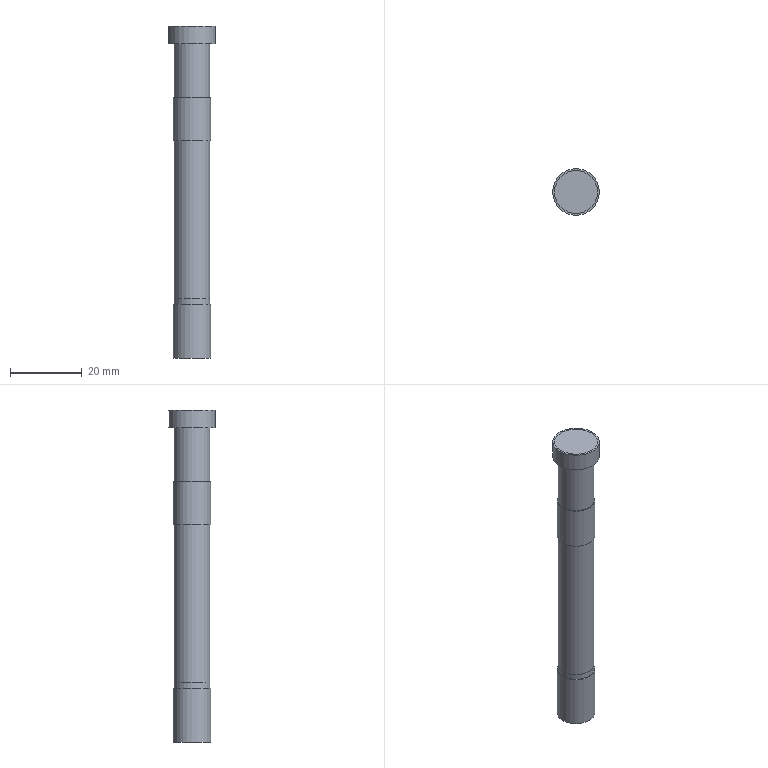Part | NX | features BREP 2 | 2 solids | 17 faces | box 13 x 13 x 92.6 mm | volume 14175 mm3 | plane 9 | cylinder 7 | cone 1 | commonest cylinder face diameters 10 x3 10.5 x2 12 x1 13 x1
STEP:
#1=CARTESIAN_POINT('',(6.5,0.,-5.));
#2=VERTEX_POINT('',#1);
#3=CARTESIAN_POINT('',(0.,0.,-5.));
#4=DIRECTION('',(0.,0.,1.));
#5=DIRECTION('',(1.,0.,0.));
#6=AXIS2_PLACEMENT_3D('',#3,#4,#5);
#7=CIRCLE('',#6,6.5);
#8=EDGE_CURVE('',#2,#2,#7,.T.);
#9=ORIENTED_EDGE('',*,*,#8,.T.);
#10=EDGE_LOOP('',(#9));
#11=FACE_BOUND('',#10,.T.);
#12=CARTESIAN_POINT('',(6.5,0.,0.));
#13=VERTEX_POINT('',#12);
#14=CARTESIAN_POINT('',(0.,0.,0.));
#15=DIRECTION('',(0.,0.,1.));
#16=DIRECTION('',(1.,0.,0.));
#17=AXIS2_PLACEMENT_3D('',#14,#15,#16);
#18=CIRCLE('',#17,6.5);
#19=EDGE_CURVE('',#13,#13,#18,.T.);
#20=ORIENTED_EDGE('',*,*,#19,.F.);
#21=EDGE_LOOP('',(#20));
#22=FACE_BOUND('',#21,.T.);
#23=CARTESIAN_POINT('',(0.,0.,-5.));
#24=DIRECTION('',(0.,0.,1.));
#25=DIRECTION('',(-1.,0.,0.));
#26=AXIS2_PLACEMENT_3D('',#23,#24,#25);
#27=CYLINDRICAL_SURFACE('',#26,6.5);
#28=ADVANCED_FACE('',(#11,#22),#27,.T.);
#29=CARTESIAN_POINT('',(-5.,0.,-5.));
#30=VERTEX_POINT('',#29);
#31=CARTESIAN_POINT('',(0.,0.,-5.));
#32=DIRECTION('',(0.,0.,-1.));
#33=DIRECTION('',(-1.,0.,0.));
#34=AXIS2_PLACEMENT_3D('',#31,#32,#33);
#35=CIRCLE('',#34,5.);
#36=EDGE_CURVE('',#30,#30,#35,.T.);
#37=ORIENTED_EDGE('',*,*,#36,.F.);
#38=EDGE_LOOP('',(#37));
#39=FACE_BOUND('',#38,.T.);
#40=ORIENTED_EDGE('',*,*,#8,.F.);
#41=EDGE_LOOP('',(#40));
#42=FACE_BOUND('',#41,.T.);
#43=CARTESIAN_POINT('',(0.,0.,-5.));
#44=DIRECTION('',(0.,0.,1.));
#45=DIRECTION('',(-1.,0.,0.));
#46=AXIS2_PLACEMENT_3D('',#43,#44,#45);
#47=PLANE('',#46);
#48=ADVANCED_FACE('',(#39,#42),#47,.F.);
#49=ORIENTED_EDGE('',*,*,#19,.T.);
#50=EDGE_LOOP('',(#49));
#51=FACE_BOUND('',#50,.T.);
#52=CARTESIAN_POINT('',(0.,0.,0.));
#53=DIRECTION('',(0.,0.,1.));
#54=DIRECTION('',(-1.,0.,0.));
#55=AXIS2_PLACEMENT_3D('',#52,#53,#54);
#56=PLANE('',#55);
#57=ADVANCED_FACE('',(#51),#56,.T.);
#58=CARTESIAN_POINT('',(-5.,0.,-20.));
#59=VERTEX_POINT('',#58);
#60=CARTESIAN_POINT('',(0.,0.,-20.));
#61=DIRECTION('',(0.,0.,-1.));
#62=DIRECTION('',(-1.,0.,0.));
#63=AXIS2_PLACEMENT_3D('',#60,#61,#62);
#64=CIRCLE('',#63,5.);
#65=EDGE_CURVE('',#59,#59,#64,.T.);
#66=ORIENTED_EDGE('',*,*,#65,.F.);
#67=EDGE_LOOP('',(#66));
#68=FACE_BOUND('',#67,.T.);
#69=ORIENTED_EDGE('',*,*,#36,.T.);
#70=EDGE_LOOP('',(#69));
#71=FACE_BOUND('',#70,.T.);
#72=CARTESIAN_POINT('',(0.,0.,-5.));
#73=DIRECTION('',(0.,0.,-1.));
#74=DIRECTION('',(1.,0.,0.));
#75=AXIS2_PLACEMENT_3D('',#72,#73,#74);
#76=CYLINDRICAL_SURFACE('',#75,5.);
#77=ADVANCED_FACE('',(#68,#71),#76,.T.);
#78=CARTESIAN_POINT('',(-5.,0.,-32.));
#79=VERTEX_POINT('',#78);
#80=CARTESIAN_POINT('',(0.,0.,-32.));
#81=DIRECTION('',(0.,0.,-1.));
#82=DIRECTION('',(-1.,0.,0.));
#83=AXIS2_PLACEMENT_3D('',#80,#81,#82);
#84=CIRCLE('',#83,5.);
#85=EDGE_CURVE('',#79,#79,#84,.T.);
#86=ORIENTED_EDGE('',*,*,#85,.F.);
#87=EDGE_LOOP('',(#86));
#88=FACE_BOUND('',#87,.T.);
#89=CARTESIAN_POINT('',(-5.25,0.,-32.));
#90=VERTEX_POINT('',#89);
#91=CARTESIAN_POINT('',(0.,0.,-32.));
#92=DIRECTION('',(0.,0.,-1.));
#93=DIRECTION('',(-1.,0.,0.));
#94=AXIS2_PLACEMENT_3D('',#91,#92,#93);
#95=CIRCLE('',#94,5.25);
#96=EDGE_CURVE('',#90,#90,#95,.T.);
#97=ORIENTED_EDGE('',*,*,#96,.T.);
#98=EDGE_LOOP('',(#97));
#99=FACE_BOUND('',#98,.T.);
#100=CARTESIAN_POINT('',(0.,0.,-32.));
#101=DIRECTION('',(0.,0.,-1.));
#102=DIRECTION('',(1.,0.,0.));
#103=AXIS2_PLACEMENT_3D('',#100,#101,#102);
#104=PLANE('',#103);
#105=ADVANCED_FACE('',(#88,#99),#104,.T.);
#106=ORIENTED_EDGE('',*,*,#65,.T.);
#107=EDGE_LOOP('',(#106));
#108=FACE_BOUND('',#107,.T.);
#109=CARTESIAN_POINT('',(-5.25,0.,-20.));
#110=VERTEX_POINT('',#109);
#111=CARTESIAN_POINT('',(0.,0.,-20.));
#112=DIRECTION('',(0.,0.,-1.));
#113=DIRECTION('',(-1.,0.,0.));
#114=AXIS2_PLACEMENT_3D('',#111,#112,#113);
#115=CIRCLE('',#114,5.25);
#116=EDGE_CURVE('',#110,#110,#115,.T.);
#117=ORIENTED_EDGE('',*,*,#116,.F.);
#118=EDGE_LOOP('',(#117));
#119=FACE_BOUND('',#118,.T.);
#120=CARTESIAN_POINT('',(0.,0.,-20.));
#121=DIRECTION('',(0.,0.,1.));
#122=DIRECTION('',(-1.,0.,0.));
#123=AXIS2_PLACEMENT_3D('',#120,#121,#122);
#124=PLANE('',#123);
#125=ADVANCED_FACE('',(#108,#119),#124,.T.);
#126=ORIENTED_EDGE('',*,*,#96,.F.);
#127=EDGE_LOOP('',(#126));
#128=FACE_BOUND('',#127,.T.);
#129=ORIENTED_EDGE('',*,*,#116,.T.);
#130=EDGE_LOOP('',(#129));
#131=FACE_BOUND('',#130,.T.);
#132=CARTESIAN_POINT('',(0.,0.,-20.));
#133=DIRECTION('',(0.,0.,-1.));
#134=DIRECTION('',(1.,0.,0.));
#135=AXIS2_PLACEMENT_3D('',#132,#133,#134);
#136=CYLINDRICAL_SURFACE('',#135,5.25);
#137=ADVANCED_FACE('',(#128,#131),#136,.T.);
#138=CARTESIAN_POINT('',(-5.,0.,-77.6));
#139=VERTEX_POINT('',#138);
#140=CARTESIAN_POINT('',(0.,0.,-77.6));
#141=DIRECTION('',(0.,0.,-1.));
#142=DIRECTION('',(-1.,0.,0.));
#143=AXIS2_PLACEMENT_3D('',#140,#141,#142);
#144=CIRCLE('',#143,5.);
#145=EDGE_CURVE('',#139,#139,#144,.T.);
#146=ORIENTED_EDGE('',*,*,#145,.F.);
#147=EDGE_LOOP('',(#146));
#148=FACE_BOUND('',#147,.T.);
#149=ORIENTED_EDGE('',*,*,#85,.T.);
#150=EDGE_LOOP('',(#149));
#151=FACE_BOUND('',#150,.T.);
#152=CARTESIAN_POINT('',(0.,0.,-32.));
#153=DIRECTION('',(0.,0.,-1.));
#154=DIRECTION('',(1.,0.,0.));
#155=AXIS2_PLACEMENT_3D('',#152,#153,#154);
#156=CYLINDRICAL_SURFACE('',#155,5.);
#157=ADVANCED_FACE('',(#148,#151),#156,.T.);
#158=CARTESIAN_POINT('',(-5.25,0.,-92.6));
#159=VERTEX_POINT('',#158);
#160=CARTESIAN_POINT('',(0.,0.,-92.6));
#161=DIRECTION('',(0.,0.,-1.));
#162=DIRECTION('',(-1.,0.,0.));
#163=AXIS2_PLACEMENT_3D('',#160,#161,#162);
#164=CIRCLE('',#163,5.25);
#165=EDGE_CURVE('',#159,#159,#164,.T.);
#166=ORIENTED_EDGE('',*,*,#165,.T.);
#167=EDGE_LOOP('',(#166));
#168=FACE_BOUND('',#167,.T.);
#169=CARTESIAN_POINT('',(0.,0.,-92.6));
#170=DIRECTION('',(0.,0.,-1.));
#171=DIRECTION('',(1.,0.,0.));
#172=AXIS2_PLACEMENT_3D('',#169,#170,#171);
#173=PLANE('',#172);
#174=ADVANCED_FACE('',(#168),#173,.T.);
#175=ORIENTED_EDGE('',*,*,#145,.T.);
#176=EDGE_LOOP('',(#175));
#177=FACE_BOUND('',#176,.T.);
#178=CARTESIAN_POINT('',(-5.25,0.,-77.6));
#179=VERTEX_POINT('',#178);
#180=CARTESIAN_POINT('',(0.,0.,-77.6));
#181=DIRECTION('',(0.,0.,-1.));
#182=DIRECTION('',(-1.,0.,0.));
#183=AXIS2_PLACEMENT_3D('',#180,#181,#182);
#184=CIRCLE('',#183,5.25);
#185=EDGE_CURVE('',#179,#179,#184,.T.);
#186=ORIENTED_EDGE('',*,*,#185,.F.);
#187=EDGE_LOOP('',(#186));
#188=FACE_BOUND('',#187,.T.);
#189=CARTESIAN_POINT('',(0.,0.,-77.6));
#190=DIRECTION('',(0.,0.,1.));
#191=DIRECTION('',(-1.,0.,0.));
#192=AXIS2_PLACEMENT_3D('',#189,#190,#191);
#193=PLANE('',#192);
#194=ADVANCED_FACE('',(#177,#188),#193,.T.);
#195=ORIENTED_EDGE('',*,*,#165,.F.);
#196=EDGE_LOOP('',(#195));
#197=FACE_BOUND('',#196,.T.);
#198=ORIENTED_EDGE('',*,*,#185,.T.);
#199=EDGE_LOOP('',(#198));
#200=FACE_BOUND('',#199,.T.);
#201=CARTESIAN_POINT('',(0.,0.,-77.6));
#202=DIRECTION('',(0.,0.,-1.));
#203=DIRECTION('',(1.,0.,0.));
#204=AXIS2_PLACEMENT_3D('',#201,#202,#203);
#205=CYLINDRICAL_SURFACE('',#204,5.25);
#206=ADVANCED_FACE('',(#197,#200),#205,.T.);
#207=CLOSED_SHELL('',(#28,#48,#57,#77,#105,#125,#137,#157,#174,#194,#206));
#208=MANIFOLD_SOLID_BREP('',#207);
#209=CARTESIAN_POINT('',(6.,0.,-5.));
#210=VERTEX_POINT('',#209);
#211=CARTESIAN_POINT('',(0.,0.,-5.));
#212=DIRECTION('',(0.,0.,1.));
#213=DIRECTION('',(1.,0.,0.));
#214=AXIS2_PLACEMENT_3D('',#211,#212,#213);
#215=CIRCLE('',#214,6.);
#216=EDGE_CURVE('',#210,#210,#215,.T.);
#217=ORIENTED_EDGE('',*,*,#216,.T.);
#218=EDGE_LOOP('',(#217));
#219=FACE_BOUND('',#218,.T.);
#220=CARTESIAN_POINT('',(6.,0.,0.));
#221=VERTEX_POINT('',#220);
#222=CARTESIAN_POINT('',(0.,0.,0.));
#223=DIRECTION('',(0.,0.,1.));
#224=DIRECTION('',(1.,0.,0.));
#225=AXIS2_PLACEMENT_3D('',#222,#223,#224);
#226=CIRCLE('',#225,6.);
#227=EDGE_CURVE('',#221,#221,#226,.T.);
#228=ORIENTED_EDGE('',*,*,#227,.F.);
#229=EDGE_LOOP('',(#228));
#230=FACE_BOUND('',#229,.T.);
#231=CARTESIAN_POINT('',(0.,0.,-5.));
#232=DIRECTION('',(0.,0.,1.));
#233=DIRECTION('',(-1.,0.,0.));
#234=AXIS2_PLACEMENT_3D('',#231,#232,#233);
#235=CYLINDRICAL_SURFACE('',#234,6.);
#236=ADVANCED_FACE('',(#219,#230),#235,.T.);
#237=CARTESIAN_POINT('',(-5.,0.,-5.));
#238=VERTEX_POINT('',#237);
#239=CARTESIAN_POINT('',(0.,0.,-5.));
#240=DIRECTION('',(0.,0.,-1.));
#241=DIRECTION('',(-1.,0.,0.));
#242=AXIS2_PLACEMENT_3D('',#239,#240,#241);
#243=CIRCLE('',#242,5.);
#244=EDGE_CURVE('',#238,#238,#243,.T.);
#245=ORIENTED_EDGE('',*,*,#244,.F.);
#246=EDGE_LOOP('',(#245));
#247=FACE_BOUND('',#246,.T.);
#248=ORIENTED_EDGE('',*,*,#216,.F.);
#249=EDGE_LOOP('',(#248));
#250=FACE_BOUND('',#249,.T.);
#251=CARTESIAN_POINT('',(0.,0.,-5.));
#252=DIRECTION('',(0.,0.,1.));
#253=DIRECTION('',(-1.,0.,0.));
#254=AXIS2_PLACEMENT_3D('',#251,#252,#253);
#255=PLANE('',#254);
#256=ADVANCED_FACE('',(#247,#250),#255,.F.);
#257=ORIENTED_EDGE('',*,*,#227,.T.);
#258=EDGE_LOOP('',(#257));
#259=FACE_BOUND('',#258,.T.);
#260=CARTESIAN_POINT('',(0.,0.,0.));
#261=DIRECTION('',(0.,0.,1.));
#262=DIRECTION('',(-1.,0.,0.));
#263=AXIS2_PLACEMENT_3D('',#260,#261,#262);
#264=PLANE('',#263);
#265=ADVANCED_FACE('',(#259),#264,.T.);
#266=CARTESIAN_POINT('',(-4.295,0.,-80.));
#267=VERTEX_POINT('',#266);
#268=CARTESIAN_POINT('',(0.,0.,-80.));
#269=DIRECTION('',(0.,0.,-1.));
#270=DIRECTION('',(-1.,0.,0.));
#271=AXIS2_PLACEMENT_3D('',#268,#269,#270);
#272=CIRCLE('',#271,4.295);
#273=EDGE_CURVE('',#267,#267,#272,.T.);
#274=ORIENTED_EDGE('',*,*,#273,.T.);
#275=EDGE_LOOP('',(#274));
#276=FACE_BOUND('',#275,.T.);
#277=CARTESIAN_POINT('',(0.,0.,-80.));
#278=DIRECTION('',(0.,0.,-1.));
#279=DIRECTION('',(1.,0.,0.));
#280=AXIS2_PLACEMENT_3D('',#277,#278,#279);
#281=PLANE('',#280);
#282=ADVANCED_FACE('',(#276),#281,.T.);
#283=CARTESIAN_POINT('',(-5.,0.,-76.));
#284=VERTEX_POINT('',#283);
#285=CARTESIAN_POINT('',(0.,0.,-76.));
#286=DIRECTION('',(0.,0.,1.));
#287=DIRECTION('',(-1.,0.,0.));
#288=AXIS2_PLACEMENT_3D('',#285,#286,#287);
#289=CIRCLE('',#288,5.);
#290=EDGE_CURVE('',#284,#284,#289,.T.);
#291=ORIENTED_EDGE('',*,*,#290,.T.);
#292=EDGE_LOOP('',(#291));
#293=FACE_BOUND('',#292,.T.);
#294=ORIENTED_EDGE('',*,*,#244,.T.);
#295=EDGE_LOOP('',(#294));
#296=FACE_BOUND('',#295,.T.);
#297=CARTESIAN_POINT('',(0.,0.,-5.));
#298=DIRECTION('',(0.,0.,-1.));
#299=DIRECTION('',(1.,0.,0.));
#300=AXIS2_PLACEMENT_3D('',#297,#298,#299);
#301=CYLINDRICAL_SURFACE('',#300,5.);
#302=ADVANCED_FACE('',(#293,#296),#301,.T.);
#303=ORIENTED_EDGE('',*,*,#290,.F.);
#304=EDGE_LOOP('',(#303));
#305=FACE_BOUND('',#304,.T.);
#306=ORIENTED_EDGE('',*,*,#273,.F.);
#307=EDGE_LOOP('',(#306));
#308=FACE_BOUND('',#307,.T.);
#309=CARTESIAN_POINT('',(0.,0.,-80.));
#310=DIRECTION('',(0.,0.,1.));
#311=DIRECTION('',(-1.,0.,0.));
#312=AXIS2_PLACEMENT_3D('',#309,#310,#311);
#313=CONICAL_SURFACE('',#312,4.295,0.1745);
#314=ADVANCED_FACE('',(#305,#308),#313,.T.);
#315=CLOSED_SHELL('',(#236,#256,#265,#282,#302,#314));
#316=MANIFOLD_SOLID_BREP('',#315);
#317=(LENGTH_UNIT()NAMED_UNIT(*)SI_UNIT(.MILLI.,.METRE.));
#318=UNCERTAINTY_MEASURE_WITH_UNIT(LENGTH_MEASURE(0.00001),#317,'','');
#319=(NAMED_UNIT(*)PLANE_ANGLE_UNIT()SI_UNIT($,.RADIAN.));
#320=(NAMED_UNIT(*)SI_UNIT($,.STERADIAN.)SOLID_ANGLE_UNIT());
#321=(GEOMETRIC_REPRESENTATION_CONTEXT(3)GLOBAL_UNCERTAINTY_ASSIGNED_CONTEXT((#318))GLOBAL_UNIT_ASSIGNED_CONTEXT((#317,#319,#320))REPRESENTATION_CONTEXT('',''));
#322=ADVANCED_BREP_SHAPE_REPRESENTATION('',(#208,#316),#321);